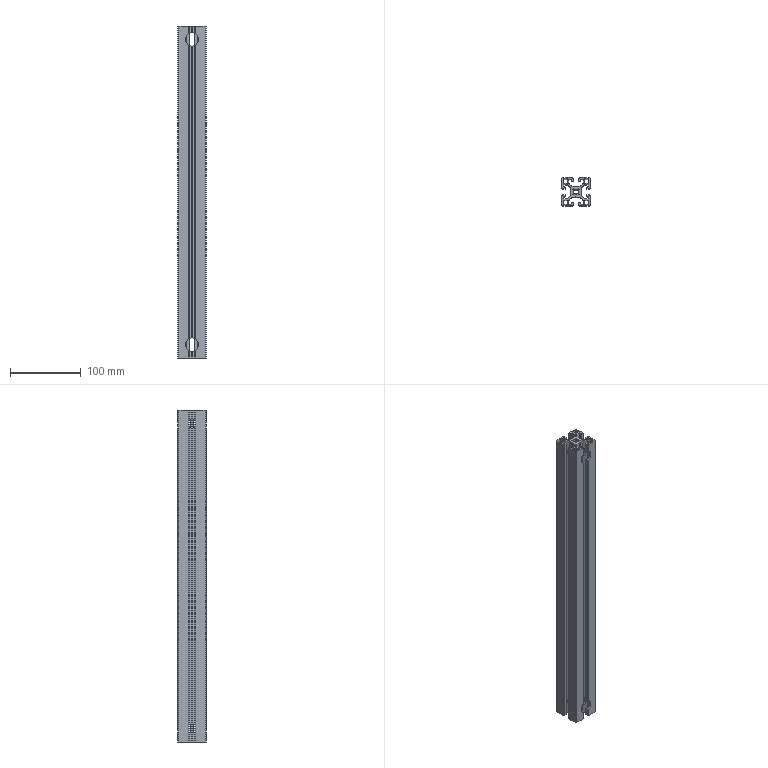Part | NX | features BREP 1 | 1 solid | 273 faces | box 40 x 40 x 470 mm | volume 278616 mm3 | plane 186 | cylinder 87 | commonest cylinder face diameters 1.5 x18 0.6 x16 2 x16 19 x16 6.8 x9 1 x8